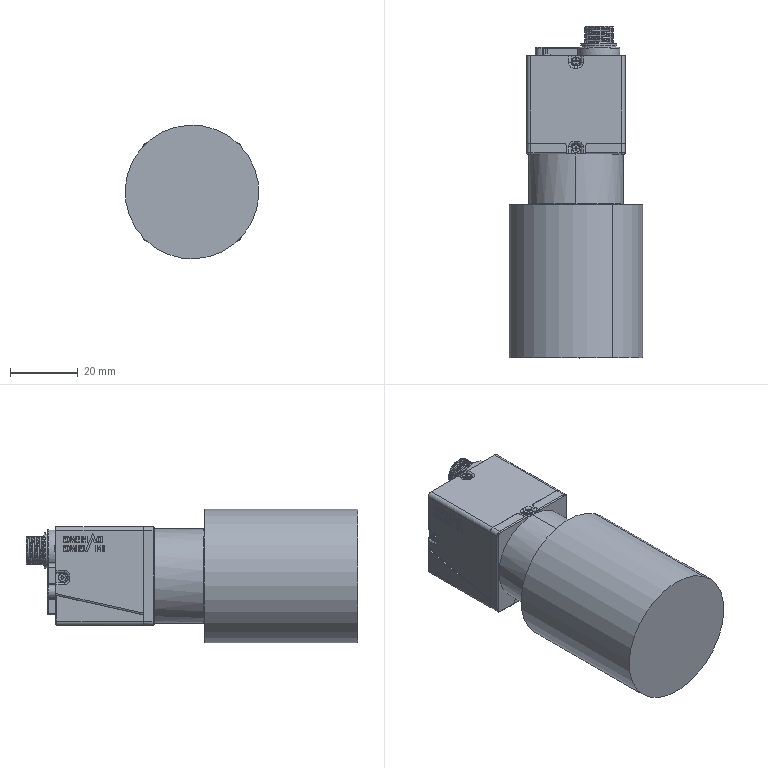Part | SolidWorks | 1 solid | 1437 faces | box 39.5 x 98.192 x 39.5 mm | volume 82462 mm3 | plane 776 | cylinder 384 | spline 171 | cone 103 | torus 3 | commonest cylinder face diameters 0.4 x84 1.4 x39 8.5 x21 2 x20 1 x17 0.6 x15